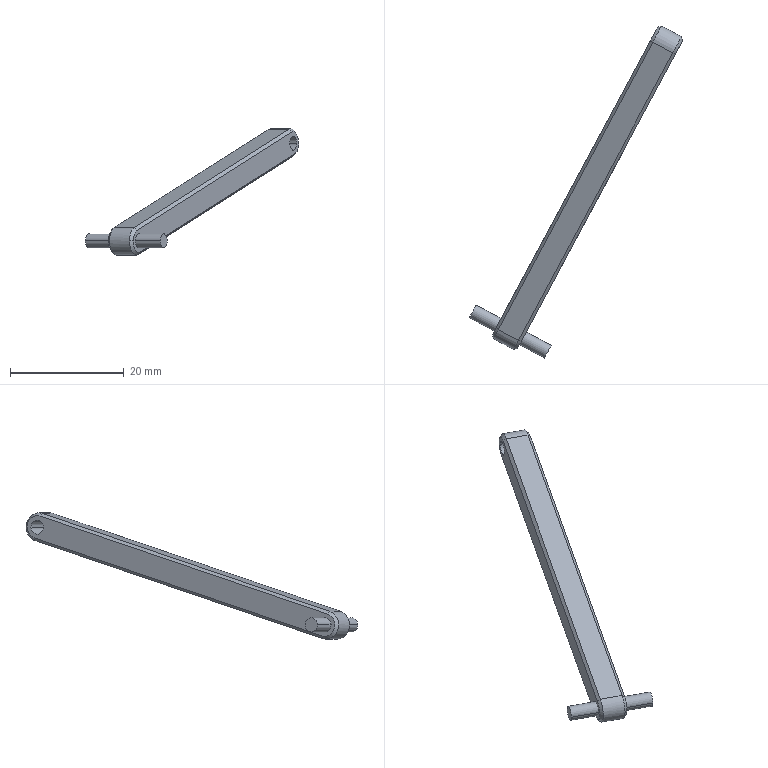Part | SolidWorks | features Revolution 2, Chamfer 1, Extrusion 1, HoleWzd 1 | 1 solid | 25 faces | box 37.545 x 58.428 x 22.236 mm | volume 1589 mm3 | plane 10 | cylinder 9 | cone 6 | commonest cylinder face diameters 2.5 x6 5 x3
STEP:
#1=CARTESIAN_POINT('',(-5.347,-33.041,-248.108));
#2=VERTEX_POINT('',#1);
#3=CARTESIAN_POINT('',(-6.022,-34.297,-250.024));
#4=VERTEX_POINT('',#3);
#5=CARTESIAN_POINT('',(-6.294,-34.803,-248.108));
#6=DIRECTION('',(-0.8809,0.4732,0.));
#7=DIRECTION('',(0.4732,0.8809,0.));
#8=AXIS2_PLACEMENT_3D('',#5,#6,#7);
#9=CIRCLE('',#8,2.);
#10=EDGE_CURVE('',#2,#4,#9,.T.);
#11=ORIENTED_EDGE('',*,*,#10,.F.);
#12=CARTESIAN_POINT('',(-4.67,-32.837,-248.108));
#13=VERTEX_POINT('',#12);
#14=CARTESIAN_POINT('',(-4.67,-32.837,-248.108));
#15=DIRECTION('',(0.9575,0.2883,0.));
#16=VECTOR('',#15,1000.);
#17=LINE('',#14,#16);
#18=EDGE_CURVE('',#2,#13,#17,.T.);
#19=ORIENTED_EDGE('',*,*,#18,.T.);
#20=CARTESIAN_POINT('',(-5.514,-34.407,-250.503));
#21=VERTEX_POINT('',#20);
#22=CARTESIAN_POINT('',(-5.853,-35.04,-248.108));
#23=DIRECTION('',(0.8809,-0.4732,0.));
#24=DIRECTION('',(0.4732,0.8809,0.));
#25=AXIS2_PLACEMENT_3D('',#22,#23,#24);
#26=CIRCLE('',#25,2.5);
#27=EDGE_CURVE('',#21,#13,#26,.T.);
#28=ORIENTED_EDGE('',*,*,#27,.F.);
#29=CARTESIAN_POINT('',(-6.022,-34.297,-250.024));
#30=DIRECTION('',(0.719,-0.1557,-0.6773));
#31=VECTOR('',#30,1000.);
#32=LINE('',#29,#31);
#33=EDGE_CURVE('',#4,#21,#32,.T.);
#34=ORIENTED_EDGE('',*,*,#33,.F.);
#35=EDGE_LOOP('',(#11,#19,#28,#34));
#36=FACE_OUTER_BOUND('',#35,.T.);
#37=CARTESIAN_POINT('',(-5.853,-35.04,-248.108));
#38=DIRECTION('',(0.8809,-0.4732,0.));
#39=DIRECTION('',(0.4732,0.8809,0.));
#40=AXIS2_PLACEMENT_3D('',#37,#38,#39);
#41=CONICAL_SURFACE('',#40,2.5,0.7854);
#42=ADVANCED_FACE('',(#36),#41,.T.);
#43=CARTESIAN_POINT('',(-30.033,-89.559,-265.344));
#44=VERTEX_POINT('',#43);
#45=CARTESIAN_POINT('',(-28.815,-87.291,-267.26));
#46=VERTEX_POINT('',#45);
#47=CARTESIAN_POINT('',(-29.087,-87.798,-265.344));
#48=DIRECTION('',(0.8809,-0.4732,0.));
#49=DIRECTION('',(0.4732,0.8809,0.));
#50=AXIS2_PLACEMENT_3D('',#47,#48,#49);
#51=CIRCLE('',#50,2.);
#52=EDGE_CURVE('',#44,#46,#51,.T.);
#53=ORIENTED_EDGE('',*,*,#52,.F.);
#54=CARTESIAN_POINT('',(-30.71,-89.763,-265.344));
#55=VERTEX_POINT('',#54);
#56=CARTESIAN_POINT('',(-30.033,-89.559,-265.344));
#57=DIRECTION('',(-0.9575,-0.2883,0.));
#58=VECTOR('',#57,1000.);
#59=LINE('',#56,#58);
#60=EDGE_CURVE('',#44,#55,#59,.T.);
#61=ORIENTED_EDGE('',*,*,#60,.T.);
#62=CARTESIAN_POINT('',(-29.187,-86.928,-267.739));
#63=VERTEX_POINT('',#62);
#64=CARTESIAN_POINT('',(-29.527,-87.561,-265.344));
#65=DIRECTION('',(-0.8809,0.4732,0.));
#66=DIRECTION('',(0.4732,0.8809,0.));
#67=AXIS2_PLACEMENT_3D('',#64,#65,#66);
#68=CIRCLE('',#67,2.5);
#69=EDGE_CURVE('',#63,#55,#68,.T.);
#70=ORIENTED_EDGE('',*,*,#69,.F.);
#71=CARTESIAN_POINT('',(-28.815,-87.291,-267.26));
#72=DIRECTION('',(-0.5268,0.5136,-0.6773));
#73=VECTOR('',#72,1000.);
#74=LINE('',#71,#73);
#75=EDGE_CURVE('',#46,#63,#74,.T.);
#76=ORIENTED_EDGE('',*,*,#75,.F.);
#77=EDGE_LOOP('',(#53,#61,#70,#76));
#78=FACE_OUTER_BOUND('',#77,.T.);
#79=CARTESIAN_POINT('',(-29.087,-87.798,-265.344));
#80=DIRECTION('',(-0.8809,0.4732,0.));
#81=DIRECTION('',(-0.4732,-0.8809,0.));
#82=AXIS2_PLACEMENT_3D('',#79,#80,#81);
#83=CONICAL_SURFACE('',#82,2.,0.7854);
#84=ADVANCED_FACE('',(#78),#83,.T.);
#85=CARTESIAN_POINT('',(-2.481,-38.27,-248.108));
#86=VERTEX_POINT('',#85);
#87=CARTESIAN_POINT('',(-1.298,-36.068,-248.108));
#88=VERTEX_POINT('',#87);
#89=CARTESIAN_POINT('',(-1.889,-37.169,-248.108));
#90=DIRECTION('',(0.8809,-0.4732,0.));
#91=DIRECTION('',(0.4732,0.8809,0.));
#92=AXIS2_PLACEMENT_3D('',#89,#90,#91);
#93=CIRCLE('',#92,1.25);
#94=EDGE_CURVE('',#86,#88,#93,.T.);
#95=ORIENTED_EDGE('',*,*,#94,.T.);
#96=CARTESIAN_POINT('',(-5.702,-33.702,-248.108));
#97=VERTEX_POINT('',#96);
#98=CARTESIAN_POINT('',(-5.702,-33.702,-248.108));
#99=DIRECTION('',(-0.8809,0.4732,0.));
#100=VECTOR('',#99,1000.);
#101=LINE('',#98,#100);
#102=EDGE_CURVE('',#88,#97,#101,.T.);
#103=ORIENTED_EDGE('',*,*,#102,.T.);
#104=CARTESIAN_POINT('',(-6.885,-35.904,-248.108));
#105=VERTEX_POINT('',#104);
#106=CARTESIAN_POINT('',(-6.294,-34.803,-248.108));
#107=DIRECTION('',(-0.8809,0.4732,0.));
#108=DIRECTION('',(-0.4732,-0.8809,0.));
#109=AXIS2_PLACEMENT_3D('',#106,#107,#108);
#110=CIRCLE('',#109,1.25);
#111=EDGE_CURVE('',#97,#105,#110,.T.);
#112=ORIENTED_EDGE('',*,*,#111,.T.);
#113=CARTESIAN_POINT('',(-6.885,-35.904,-248.108));
#114=DIRECTION('',(-0.8809,0.4732,0.));
#115=VECTOR('',#114,1000.);
#116=LINE('',#113,#115);
#117=EDGE_CURVE('',#86,#105,#116,.T.);
#118=ORIENTED_EDGE('',*,*,#117,.F.);
#119=EDGE_LOOP('',(#95,#103,#112,#118));
#120=FACE_OUTER_BOUND('',#119,.T.);
#121=CARTESIAN_POINT('',(-6.294,-34.803,-248.108));
#122=DIRECTION('',(-0.8809,0.4732,0.));
#123=DIRECTION('',(-0.4732,-0.8809,0.));
#124=AXIS2_PLACEMENT_3D('',#121,#122,#123);
#125=CYLINDRICAL_SURFACE('',#124,1.25);
#126=ADVANCED_FACE('',(#120),#125,.F.);
#127=CARTESIAN_POINT('',(-28.495,-86.696,-265.344));
#128=VERTEX_POINT('',#127);
#129=CARTESIAN_POINT('',(-29.678,-88.899,-265.344));
#130=VERTEX_POINT('',#129);
#131=CARTESIAN_POINT('',(-29.087,-87.798,-265.344));
#132=DIRECTION('',(0.8809,-0.4732,0.));
#133=DIRECTION('',(0.4732,0.8809,0.));
#134=AXIS2_PLACEMENT_3D('',#131,#132,#133);
#135=CIRCLE('',#134,1.25);
#136=EDGE_CURVE('',#128,#130,#135,.T.);
#137=ORIENTED_EDGE('',*,*,#136,.T.);
#138=CARTESIAN_POINT('',(-25.274,-91.265,-265.344));
#139=VERTEX_POINT('',#138);
#140=CARTESIAN_POINT('',(-28.692,-89.429,-265.344));
#141=DIRECTION('',(0.8809,-0.4732,0.));
#142=VECTOR('',#141,1000.);
#143=LINE('',#140,#142);
#144=EDGE_CURVE('',#130,#139,#143,.T.);
#145=ORIENTED_EDGE('',*,*,#144,.T.);
#146=CARTESIAN_POINT('',(-24.09,-89.063,-265.344));
#147=VERTEX_POINT('',#146);
#148=CARTESIAN_POINT('',(-24.682,-90.164,-265.344));
#149=DIRECTION('',(0.8809,-0.4732,0.));
#150=DIRECTION('',(0.4732,0.8809,0.));
#151=AXIS2_PLACEMENT_3D('',#148,#149,#150);
#152=CIRCLE('',#151,1.25);
#153=EDGE_CURVE('',#147,#139,#152,.T.);
#154=ORIENTED_EDGE('',*,*,#153,.F.);
#155=CARTESIAN_POINT('',(-27.509,-87.226,-265.344));
#156=DIRECTION('',(0.8809,-0.4732,0.));
#157=VECTOR('',#156,1000.);
#158=LINE('',#155,#157);
#159=EDGE_CURVE('',#128,#147,#158,.T.);
#160=ORIENTED_EDGE('',*,*,#159,.F.);
#161=EDGE_LOOP('',(#137,#145,#154,#160));
#162=FACE_OUTER_BOUND('',#161,.T.);
#163=CARTESIAN_POINT('',(-28.1,-88.327,-265.344));
#164=DIRECTION('',(0.8809,-0.4732,0.));
#165=DIRECTION('',(0.4732,0.8809,0.));
#166=AXIS2_PLACEMENT_3D('',#163,#164,#165);
#167=CYLINDRICAL_SURFACE('',#166,1.25);
#168=ADVANCED_FACE('',(#162),#167,.T.);
#169=CARTESIAN_POINT('',(-37.304,-81.964,-265.344));
#170=VERTEX_POINT('',#169);
#171=CARTESIAN_POINT('',(-38.488,-84.166,-265.344));
#172=VERTEX_POINT('',#171);
#173=CARTESIAN_POINT('',(-37.896,-83.065,-265.344));
#174=DIRECTION('',(0.8809,-0.4732,0.));
#175=DIRECTION('',(0.4732,0.8809,0.));
#176=AXIS2_PLACEMENT_3D('',#173,#174,#175);
#177=CIRCLE('',#176,1.25);
#178=EDGE_CURVE('',#170,#172,#177,.T.);
#179=ORIENTED_EDGE('',*,*,#178,.T.);
#180=CARTESIAN_POINT('',(-34.083,-86.532,-265.344));
#181=VERTEX_POINT('',#180);
#182=CARTESIAN_POINT('',(-37.501,-84.696,-265.344));
#183=DIRECTION('',(0.8809,-0.4732,0.));
#184=VECTOR('',#183,1000.);
#185=LINE('',#182,#184);
#186=EDGE_CURVE('',#172,#181,#185,.T.);
#187=ORIENTED_EDGE('',*,*,#186,.T.);
#188=CARTESIAN_POINT('',(-32.9,-84.33,-265.344));
#189=VERTEX_POINT('',#188);
#190=CARTESIAN_POINT('',(-33.491,-85.431,-265.344));
#191=DIRECTION('',(0.8809,-0.4732,0.));
#192=DIRECTION('',(0.4732,0.8809,0.));
#193=AXIS2_PLACEMENT_3D('',#190,#191,#192);
#194=CIRCLE('',#193,1.25);
#195=EDGE_CURVE('',#189,#181,#194,.T.);
#196=ORIENTED_EDGE('',*,*,#195,.F.);
#197=CARTESIAN_POINT('',(-36.318,-82.494,-265.344));
#198=DIRECTION('',(0.8809,-0.4732,0.));
#199=VECTOR('',#198,1000.);
#200=LINE('',#197,#199);
#201=EDGE_CURVE('',#170,#189,#200,.T.);
#202=ORIENTED_EDGE('',*,*,#201,.F.);
#203=EDGE_LOOP('',(#179,#187,#196,#202));
#204=FACE_OUTER_BOUND('',#203,.T.);
#205=CARTESIAN_POINT('',(-36.91,-83.595,-265.344));
#206=DIRECTION('',(0.8809,-0.4732,0.));
#207=DIRECTION('',(0.4732,0.8809,0.));
#208=AXIS2_PLACEMENT_3D('',#205,#206,#207);
#209=CYLINDRICAL_SURFACE('',#208,1.25);
#210=ADVANCED_FACE('',(#204),#209,.T.);
#211=ORIENTED_EDGE('',*,*,#27,.T.);
#212=CARTESIAN_POINT('',(-1.147,-34.73,-248.108));
#213=VERTEX_POINT('',#212);
#214=CARTESIAN_POINT('',(-5.111,-32.601,-248.108));
#215=DIRECTION('',(0.8809,-0.4732,0.));
#216=VECTOR('',#215,1000.);
#217=LINE('',#214,#216);
#218=EDGE_CURVE('',#13,#213,#217,.T.);
#219=ORIENTED_EDGE('',*,*,#218,.T.);
#220=CARTESIAN_POINT('',(-1.99,-36.3,-250.503));
#221=VERTEX_POINT('',#220);
#222=CARTESIAN_POINT('',(-2.33,-36.933,-248.108));
#223=DIRECTION('',(-0.8809,0.4732,0.));
#224=DIRECTION('',(0.4732,0.8809,0.));
#225=AXIS2_PLACEMENT_3D('',#222,#223,#224);
#226=CIRCLE('',#225,2.5);
#227=EDGE_CURVE('',#213,#221,#226,.T.);
#228=ORIENTED_EDGE('',*,*,#227,.T.);
#229=CARTESIAN_POINT('',(-5.954,-34.17,-250.503));
#230=DIRECTION('',(0.8809,-0.4732,0.));
#231=VECTOR('',#230,1000.);
#232=LINE('',#229,#231);
#233=EDGE_CURVE('',#21,#221,#232,.T.);
#234=ORIENTED_EDGE('',*,*,#233,.F.);
#235=EDGE_LOOP('',(#211,#219,#228,#234));
#236=FACE_OUTER_BOUND('',#235,.T.);
#237=CARTESIAN_POINT('',(-6.294,-34.803,-248.108));
#238=DIRECTION('',(0.8809,-0.4732,0.));
#239=DIRECTION('',(0.4732,0.8809,0.));
#240=AXIS2_PLACEMENT_3D('',#237,#238,#239);
#241=CYLINDRICAL_SURFACE('',#240,2.5);
#242=ADVANCED_FACE('',(#236),#241,.T.);
#243=CARTESIAN_POINT('',(-32.711,-85.035,-267.739));
#244=VERTEX_POINT('',#243);
#245=CARTESIAN_POINT('',(-33.151,-84.799,-267.739));
#246=DIRECTION('',(0.8809,-0.4732,0.));
#247=VECTOR('',#246,1000.);
#248=LINE('',#245,#247);
#249=EDGE_CURVE('',#244,#63,#248,.T.);
#250=ORIENTED_EDGE('',*,*,#249,.T.);
#251=ORIENTED_EDGE('',*,*,#69,.T.);
#252=CARTESIAN_POINT('',(-29.867,-88.194,-262.949));
#253=VERTEX_POINT('',#252);
#254=CARTESIAN_POINT('',(-29.527,-87.561,-265.344));
#255=DIRECTION('',(-0.8809,0.4732,0.));
#256=DIRECTION('',(0.4732,0.8809,0.));
#257=AXIS2_PLACEMENT_3D('',#254,#255,#256);
#258=CIRCLE('',#257,2.5);
#259=EDGE_CURVE('',#55,#253,#258,.T.);
#260=ORIENTED_EDGE('',*,*,#259,.T.);
#261=CARTESIAN_POINT('',(-33.391,-86.301,-262.949));
#262=VERTEX_POINT('',#261);
#263=CARTESIAN_POINT('',(-33.831,-86.064,-262.949));
#264=DIRECTION('',(0.8809,-0.4732,0.));
#265=VECTOR('',#264,1000.);
#266=LINE('',#263,#265);
#267=EDGE_CURVE('',#262,#253,#266,.T.);
#268=ORIENTED_EDGE('',*,*,#267,.F.);
#269=CARTESIAN_POINT('',(-33.051,-85.668,-265.344));
#270=DIRECTION('',(0.8809,-0.4732,0.));
#271=DIRECTION('',(0.4732,0.8809,0.));
#272=AXIS2_PLACEMENT_3D('',#269,#270,#271);
#273=CIRCLE('',#272,2.5);
#274=EDGE_CURVE('',#262,#244,#273,.T.);
#275=ORIENTED_EDGE('',*,*,#274,.T.);
#276=EDGE_LOOP('',(#250,#251,#260,#268,#275));
#277=FACE_OUTER_BOUND('',#276,.T.);
#278=CARTESIAN_POINT('',(-33.491,-85.431,-265.344));
#279=DIRECTION('',(0.8809,-0.4732,0.));
#280=DIRECTION('',(0.4732,0.8809,0.));
#281=AXIS2_PLACEMENT_3D('',#278,#279,#280);
#282=CYLINDRICAL_SURFACE('',#281,2.5);
#283=ADVANCED_FACE('',(#277),#282,.T.);
#284=ORIENTED_EDGE('',*,*,#267,.T.);
#285=CARTESIAN_POINT('',(-2.67,-37.565,-245.714));
#286=VERTEX_POINT('',#285);
#287=CARTESIAN_POINT('',(-2.67,-37.565,-245.714));
#288=DIRECTION('',(0.4533,0.8438,0.2873));
#289=VECTOR('',#288,1000.);
#290=LINE('',#287,#289);
#291=EDGE_CURVE('',#253,#286,#290,.T.);
#292=ORIENTED_EDGE('',*,*,#291,.T.);
#293=CARTESIAN_POINT('',(-6.193,-35.672,-245.714));
#294=VERTEX_POINT('',#293);
#295=CARTESIAN_POINT('',(-6.634,-35.436,-245.714));
#296=DIRECTION('',(0.8809,-0.4732,0.));
#297=VECTOR('',#296,1000.);
#298=LINE('',#295,#297);
#299=EDGE_CURVE('',#294,#286,#298,.T.);
#300=ORIENTED_EDGE('',*,*,#299,.F.);
#301=CARTESIAN_POINT('',(-33.391,-86.301,-262.949));
#302=DIRECTION('',(-0.4533,-0.8438,-0.2873));
#303=VECTOR('',#302,1000.);
#304=LINE('',#301,#303);
#305=EDGE_CURVE('',#294,#262,#304,.T.);
#306=ORIENTED_EDGE('',*,*,#305,.T.);
#307=EDGE_LOOP('',(#284,#292,#300,#306));
#308=FACE_OUTER_BOUND('',#307,.T.);
#309=CARTESIAN_POINT('',(-6.634,-35.436,-245.714));
#310=DIRECTION('',(-0.1359,-0.2531,0.9579));
#311=DIRECTION('',(0.,-0.9668,-0.2554));
#312=AXIS2_PLACEMENT_3D('',#309,#310,#311);
#313=PLANE('',#312);
#314=ADVANCED_FACE('',(#308),#313,.T.);
#315=ORIENTED_EDGE('',*,*,#218,.F.);
#316=CARTESIAN_POINT('',(-5.853,-35.04,-248.108));
#317=DIRECTION('',(0.8809,-0.4732,0.));
#318=DIRECTION('',(0.4732,0.8809,0.));
#319=AXIS2_PLACEMENT_3D('',#316,#317,#318);
#320=CIRCLE('',#319,2.5);
#321=EDGE_CURVE('',#13,#294,#320,.T.);
#322=ORIENTED_EDGE('',*,*,#321,.T.);
#323=ORIENTED_EDGE('',*,*,#299,.T.);
#324=CARTESIAN_POINT('',(-2.33,-36.933,-248.108));
#325=DIRECTION('',(-0.8809,0.4732,0.));
#326=DIRECTION('',(0.4732,0.8809,0.));
#327=AXIS2_PLACEMENT_3D('',#324,#325,#326);
#328=CIRCLE('',#327,2.5);
#329=EDGE_CURVE('',#286,#213,#328,.T.);
#330=ORIENTED_EDGE('',*,*,#329,.T.);
#331=EDGE_LOOP('',(#315,#322,#323,#330));
#332=FACE_OUTER_BOUND('',#331,.T.);
#333=CARTESIAN_POINT('',(-6.294,-34.803,-248.108));
#334=DIRECTION('',(0.8809,-0.4732,0.));
#335=DIRECTION('',(0.4732,0.8809,0.));
#336=AXIS2_PLACEMENT_3D('',#333,#334,#335);
#337=CYLINDRICAL_SURFACE('',#336,2.5);
#338=ADVANCED_FACE('',(#332),#337,.T.);
#339=ORIENTED_EDGE('',*,*,#233,.T.);
#340=CARTESIAN_POINT('',(-29.187,-86.928,-267.739));
#341=DIRECTION('',(-0.4533,-0.8438,-0.2873));
#342=VECTOR('',#341,1000.);
#343=LINE('',#340,#342);
#344=EDGE_CURVE('',#221,#63,#343,.T.);
#345=ORIENTED_EDGE('',*,*,#344,.T.);
#346=ORIENTED_EDGE('',*,*,#249,.F.);
#347=CARTESIAN_POINT('',(-5.514,-34.407,-250.503));
#348=DIRECTION('',(0.4533,0.8438,0.2873));
#349=VECTOR('',#348,1000.);
#350=LINE('',#347,#349);
#351=EDGE_CURVE('',#244,#21,#350,.T.);
#352=ORIENTED_EDGE('',*,*,#351,.T.);
#353=EDGE_LOOP('',(#339,#345,#346,#352));
#354=FACE_OUTER_BOUND('',#353,.T.);
#355=CARTESIAN_POINT('',(-33.151,-84.799,-267.739));
#356=DIRECTION('',(0.1359,0.2531,-0.9579));
#357=DIRECTION('',(0.,0.9668,0.2554));
#358=AXIS2_PLACEMENT_3D('',#355,#356,#357);
#359=PLANE('',#358);
#360=ADVANCED_FACE('',(#354),#359,.T.);
#361=CARTESIAN_POINT('',(-6.566,-35.309,-246.192));
#362=VERTEX_POINT('',#361);
#363=CARTESIAN_POINT('',(-6.294,-34.803,-248.108));
#364=DIRECTION('',(-0.8809,0.4732,0.));
#365=DIRECTION('',(0.4732,0.8809,0.));
#366=AXIS2_PLACEMENT_3D('',#363,#364,#365);
#367=CIRCLE('',#366,2.);
#368=EDGE_CURVE('',#362,#2,#367,.T.);
#369=ORIENTED_EDGE('',*,*,#368,.T.);
#370=ORIENTED_EDGE('',*,*,#10,.T.);
#371=CARTESIAN_POINT('',(-33.219,-84.925,-267.26));
#372=VERTEX_POINT('',#371);
#373=CARTESIAN_POINT('',(-33.219,-84.925,-267.26));
#374=DIRECTION('',(-0.4533,-0.8438,-0.2873));
#375=VECTOR('',#374,1000.);
#376=LINE('',#373,#375);
#377=EDGE_CURVE('',#4,#372,#376,.T.);
#378=ORIENTED_EDGE('',*,*,#377,.T.);
#379=CARTESIAN_POINT('',(-33.763,-85.937,-263.428));
#380=VERTEX_POINT('',#379);
#381=CARTESIAN_POINT('',(-33.491,-85.431,-265.344));
#382=DIRECTION('',(-0.8809,0.4732,0.));
#383=DIRECTION('',(0.4732,0.8809,0.));
#384=AXIS2_PLACEMENT_3D('',#381,#382,#383);
#385=CIRCLE('',#384,2.);
#386=EDGE_CURVE('',#372,#380,#385,.T.);
#387=ORIENTED_EDGE('',*,*,#386,.T.);
#388=CARTESIAN_POINT('',(-6.566,-35.309,-246.192));
#389=DIRECTION('',(0.4533,0.8438,0.2873));
#390=VECTOR('',#389,1000.);
#391=LINE('',#388,#390);
#392=EDGE_CURVE('',#380,#362,#391,.T.);
#393=ORIENTED_EDGE('',*,*,#392,.T.);
#394=EDGE_LOOP('',(#369,#370,#378,#387,#393));
#395=FACE_OUTER_BOUND('',#394,.T.);
#396=CARTESIAN_POINT('',(-6.294,-34.803,-248.108));
#397=DIRECTION('',(-0.8809,0.4732,0.));
#398=DIRECTION('',(-0.4732,-0.8809,0.));
#399=AXIS2_PLACEMENT_3D('',#396,#397,#398);
#400=CIRCLE('',#399,1.25);
#401=EDGE_CURVE('',#105,#97,#400,.T.);
#402=ORIENTED_EDGE('',*,*,#401,.F.);
#403=ORIENTED_EDGE('',*,*,#111,.F.);
#404=EDGE_LOOP('',(#402,#403));
#405=FACE_BOUND('',#404,.T.);
#406=ORIENTED_EDGE('',*,*,#195,.T.);
#407=CARTESIAN_POINT('',(-33.491,-85.431,-265.344));
#408=DIRECTION('',(0.8809,-0.4732,0.));
#409=DIRECTION('',(0.4732,0.8809,0.));
#410=AXIS2_PLACEMENT_3D('',#407,#408,#409);
#411=CIRCLE('',#410,1.25);
#412=EDGE_CURVE('',#181,#189,#411,.T.);
#413=ORIENTED_EDGE('',*,*,#412,.T.);
#414=EDGE_LOOP('',(#406,#413));
#415=FACE_BOUND('',#414,.T.);
#416=CARTESIAN_POINT('',(-33.491,-85.431,-265.344));
#417=DIRECTION('',(0.8809,-0.4732,0.));
#418=DIRECTION('',(0.4732,0.8809,0.));
#419=AXIS2_PLACEMENT_3D('',#416,#417,#418);
#420=PLANE('',#419);
#421=ADVANCED_FACE('',(#395,#405,#415),#420,.F.);
#422=CARTESIAN_POINT('',(-1.617,-36.663,-250.024));
#423=VERTEX_POINT('',#422);
#424=CARTESIAN_POINT('',(-28.815,-87.291,-267.26));
#425=DIRECTION('',(0.4533,0.8438,0.2873));
#426=VECTOR('',#425,1000.);
#427=LINE('',#424,#426);
#428=EDGE_CURVE('',#46,#423,#427,.T.);
#429=ORIENTED_EDGE('',*,*,#428,.T.);
#430=CARTESIAN_POINT('',(-2.161,-37.675,-246.192));
#431=VERTEX_POINT('',#430);
#432=CARTESIAN_POINT('',(-1.889,-37.169,-248.108));
#433=DIRECTION('',(0.8809,-0.4732,0.));
#434=DIRECTION('',(0.4732,0.8809,0.));
#435=AXIS2_PLACEMENT_3D('',#432,#433,#434);
#436=CIRCLE('',#435,2.);
#437=EDGE_CURVE('',#423,#431,#436,.T.);
#438=ORIENTED_EDGE('',*,*,#437,.T.);
#439=CARTESIAN_POINT('',(-29.359,-88.304,-263.428));
#440=VERTEX_POINT('',#439);
#441=CARTESIAN_POINT('',(-29.359,-88.304,-263.428));
#442=DIRECTION('',(-0.4533,-0.8438,-0.2873));
#443=VECTOR('',#442,1000.);
#444=LINE('',#441,#443);
#445=EDGE_CURVE('',#431,#440,#444,.T.);
#446=ORIENTED_EDGE('',*,*,#445,.T.);
#447=CARTESIAN_POINT('',(-29.087,-87.798,-265.344));
#448=DIRECTION('',(0.8809,-0.4732,0.));
#449=DIRECTION('',(0.4732,0.8809,0.));
#450=AXIS2_PLACEMENT_3D('',#447,#448,#449);
#451=CIRCLE('',#450,2.);
#452=EDGE_CURVE('',#440,#44,#451,.T.);
#453=ORIENTED_EDGE('',*,*,#452,.T.);
#454=ORIENTED_EDGE('',*,*,#52,.T.);
#455=EDGE_LOOP('',(#429,#438,#446,#453,#454));
#456=FACE_OUTER_BOUND('',#455,.T.);
#457=ORIENTED_EDGE('',*,*,#94,.F.);
#458=CARTESIAN_POINT('',(-1.889,-37.169,-248.108));
#459=DIRECTION('',(0.8809,-0.4732,0.));
#460=DIRECTION('',(0.4732,0.8809,0.));
#461=AXIS2_PLACEMENT_3D('',#458,#459,#460);
#462=CIRCLE('',#461,1.25);
#463=EDGE_CURVE('',#88,#86,#462,.T.);
#464=ORIENTED_EDGE('',*,*,#463,.F.);
#465=EDGE_LOOP('',(#457,#464));
#466=FACE_BOUND('',#465,.T.);
#467=ORIENTED_EDGE('',*,*,#136,.F.);
#468=CARTESIAN_POINT('',(-29.087,-87.798,-265.344));
#469=DIRECTION('',(0.8809,-0.4732,0.));
#470=DIRECTION('',(0.4732,0.8809,0.));
#471=AXIS2_PLACEMENT_3D('',#468,#469,#470);
#472=CIRCLE('',#471,1.25);
#473=EDGE_CURVE('',#130,#128,#472,.T.);
#474=ORIENTED_EDGE('',*,*,#473,.F.);
#475=EDGE_LOOP('',(#467,#474));
#476=FACE_BOUND('',#475,.T.);
#477=CARTESIAN_POINT('',(-29.087,-87.798,-265.344));
#478=DIRECTION('',(0.8809,-0.4732,0.));
#479=DIRECTION('',(0.4732,0.8809,0.));
#480=AXIS2_PLACEMENT_3D('',#477,#478,#479);
#481=PLANE('',#480);
#482=ADVANCED_FACE('',(#456,#466,#476),#481,.T.);
#483=ORIENTED_EDGE('',*,*,#186,.F.);
#484=CARTESIAN_POINT('',(-37.896,-83.065,-265.344));
#485=DIRECTION('',(0.8809,-0.4732,0.));
#486=DIRECTION('',(0.4732,0.8809,0.));
#487=AXIS2_PLACEMENT_3D('',#484,#485,#486);
#488=CIRCLE('',#487,1.25);
#489=EDGE_CURVE('',#172,#170,#488,.T.);
#490=ORIENTED_EDGE('',*,*,#489,.T.);
#491=ORIENTED_EDGE('',*,*,#201,.T.);
#492=ORIENTED_EDGE('',*,*,#412,.F.);
#493=EDGE_LOOP('',(#483,#490,#491,#492));
#494=FACE_OUTER_BOUND('',#493,.T.);
#495=CARTESIAN_POINT('',(-36.91,-83.595,-265.344));
#496=DIRECTION('',(0.8809,-0.4732,0.));
#497=DIRECTION('',(0.4732,0.8809,0.));
#498=AXIS2_PLACEMENT_3D('',#495,#496,#497);
#499=CYLINDRICAL_SURFACE('',#498,1.25);
#500=ADVANCED_FACE('',(#494),#499,.T.);
#501=ORIENTED_EDGE('',*,*,#178,.F.);
#502=ORIENTED_EDGE('',*,*,#489,.F.);
#503=EDGE_LOOP('',(#501,#502));
#504=FACE_OUTER_BOUND('',#503,.T.);
#505=CARTESIAN_POINT('',(-37.304,-81.964,-265.344));
#506=DIRECTION('',(-0.8809,0.4732,0.));
#507=DIRECTION('',(-0.4732,-0.8809,0.));
#508=AXIS2_PLACEMENT_3D('',#505,#506,#507);
#509=PLANE('',#508);
#510=ADVANCED_FACE('',(#504),#509,.T.);
#511=ORIENTED_EDGE('',*,*,#144,.F.);
#512=ORIENTED_EDGE('',*,*,#473,.T.);
#513=ORIENTED_EDGE('',*,*,#159,.T.);
#514=CARTESIAN_POINT('',(-24.682,-90.164,-265.344));
#515=DIRECTION('',(0.8809,-0.4732,0.));
#516=DIRECTION('',(0.4732,0.8809,0.));
#517=AXIS2_PLACEMENT_3D('',#514,#515,#516);
#518=CIRCLE('',#517,1.25);
#519=EDGE_CURVE('',#139,#147,#518,.T.);
#520=ORIENTED_EDGE('',*,*,#519,.F.);
#521=EDGE_LOOP('',(#511,#512,#513,#520));
#522=FACE_OUTER_BOUND('',#521,.T.);
#523=CARTESIAN_POINT('',(-28.1,-88.327,-265.344));
#524=DIRECTION('',(0.8809,-0.4732,0.));
#525=DIRECTION('',(0.4732,0.8809,0.));
#526=AXIS2_PLACEMENT_3D('',#523,#524,#525);
#527=CYLINDRICAL_SURFACE('',#526,1.25);
#528=ADVANCED_FACE('',(#522),#527,.T.);
#529=ORIENTED_EDGE('',*,*,#153,.T.);
#530=ORIENTED_EDGE('',*,*,#519,.T.);
#531=EDGE_LOOP('',(#529,#530));
#532=FACE_OUTER_BOUND('',#531,.T.);
#533=CARTESIAN_POINT('',(-24.682,-90.164,-265.344));
#534=DIRECTION('',(0.8809,-0.4732,0.));
#535=DIRECTION('',(0.4732,0.8809,0.));
#536=AXIS2_PLACEMENT_3D('',#533,#534,#535);
#537=PLANE('',#536);
#538=ADVANCED_FACE('',(#532),#537,.T.);
#539=ORIENTED_EDGE('',*,*,#102,.F.);
#540=ORIENTED_EDGE('',*,*,#463,.T.);
#541=ORIENTED_EDGE('',*,*,#117,.T.);
#542=ORIENTED_EDGE('',*,*,#401,.T.);
#543=EDGE_LOOP('',(#539,#540,#541,#542));
#544=FACE_OUTER_BOUND('',#543,.T.);
#545=CARTESIAN_POINT('',(-6.294,-34.803,-248.108));
#546=DIRECTION('',(-0.8809,0.4732,0.));
#547=DIRECTION('',(-0.4732,-0.8809,0.));
#548=AXIS2_PLACEMENT_3D('',#545,#546,#547);
#549=CYLINDRICAL_SURFACE('',#548,1.25);
#550=ADVANCED_FACE('',(#544),#549,.F.);
#551=ORIENTED_EDGE('',*,*,#60,.F.);
#552=ORIENTED_EDGE('',*,*,#452,.F.);
#553=CARTESIAN_POINT('',(-29.867,-88.194,-262.949));
#554=DIRECTION('',(0.719,-0.1557,-0.6773));
#555=VECTOR('',#554,1000.);
#556=LINE('',#553,#555);
#557=EDGE_CURVE('',#253,#440,#556,.T.);
#558=ORIENTED_EDGE('',*,*,#557,.F.);
#559=ORIENTED_EDGE('',*,*,#259,.F.);
#560=EDGE_LOOP('',(#551,#552,#558,#559));
#561=FACE_OUTER_BOUND('',#560,.T.);
#562=CARTESIAN_POINT('',(-29.087,-87.798,-265.344));
#563=DIRECTION('',(-0.8809,0.4732,0.));
#564=DIRECTION('',(-0.4732,-0.8809,0.));
#565=AXIS2_PLACEMENT_3D('',#562,#563,#564);
#566=CONICAL_SURFACE('',#565,2.,0.7854);
#567=ADVANCED_FACE('',(#561),#566,.T.);
#568=ORIENTED_EDGE('',*,*,#75,.T.);
#569=ORIENTED_EDGE('',*,*,#344,.F.);
#570=CARTESIAN_POINT('',(-1.617,-36.663,-250.024));
#571=DIRECTION('',(-0.5268,0.5136,-0.6773));
#572=VECTOR('',#571,1000.);
#573=LINE('',#570,#572);
#574=EDGE_CURVE('',#423,#221,#573,.T.);
#575=ORIENTED_EDGE('',*,*,#574,.F.);
#576=ORIENTED_EDGE('',*,*,#428,.F.);
#577=EDGE_LOOP('',(#568,#569,#575,#576));
#578=FACE_OUTER_BOUND('',#577,.T.);
#579=CARTESIAN_POINT('',(-28.815,-87.291,-267.26));
#580=DIRECTION('',(-0.719,0.1557,0.6773));
#581=DIRECTION('',(0.4533,0.8438,0.2873));
#582=AXIS2_PLACEMENT_3D('',#579,#580,#581);
#583=PLANE('',#582);
#584=ADVANCED_FACE('',(#578),#583,.F.);
#585=ORIENTED_EDGE('',*,*,#557,.T.);
#586=ORIENTED_EDGE('',*,*,#445,.F.);
#587=CARTESIAN_POINT('',(-2.67,-37.565,-245.714));
#588=DIRECTION('',(0.719,-0.1557,-0.6773));
#589=VECTOR('',#588,1000.);
#590=LINE('',#587,#589);
#591=EDGE_CURVE('',#286,#431,#590,.T.);
#592=ORIENTED_EDGE('',*,*,#591,.F.);
#593=ORIENTED_EDGE('',*,*,#291,.F.);
#594=EDGE_LOOP('',(#585,#586,#592,#593));
#595=FACE_OUTER_BOUND('',#594,.T.);
#596=CARTESIAN_POINT('',(-29.359,-88.304,-263.428));
#597=DIRECTION('',(-0.5268,0.5136,-0.6773));
#598=DIRECTION('',(-0.4533,-0.8438,-0.2873));
#599=AXIS2_PLACEMENT_3D('',#596,#597,#598);
#600=PLANE('',#599);
#601=ADVANCED_FACE('',(#595),#600,.F.);
#602=ORIENTED_EDGE('',*,*,#574,.T.);
#603=ORIENTED_EDGE('',*,*,#227,.F.);
#604=ORIENTED_EDGE('',*,*,#329,.F.);
#605=ORIENTED_EDGE('',*,*,#591,.T.);
#606=ORIENTED_EDGE('',*,*,#437,.F.);
#607=EDGE_LOOP('',(#602,#603,#604,#605,#606));
#608=FACE_OUTER_BOUND('',#607,.T.);
#609=CARTESIAN_POINT('',(-1.889,-37.169,-248.108));
#610=DIRECTION('',(-0.8809,0.4732,0.));
#611=DIRECTION('',(-0.4732,-0.8809,0.));
#612=AXIS2_PLACEMENT_3D('',#609,#610,#611);
#613=CONICAL_SURFACE('',#612,2.,0.7854);
#614=ADVANCED_FACE('',(#608),#613,.T.);
#615=CARTESIAN_POINT('',(-6.566,-35.309,-246.192));
#616=DIRECTION('',(0.5268,-0.5136,0.6773));
#617=VECTOR('',#616,1000.);
#618=LINE('',#615,#617);
#619=EDGE_CURVE('',#362,#294,#618,.T.);
#620=ORIENTED_EDGE('',*,*,#619,.F.);
#621=ORIENTED_EDGE('',*,*,#392,.F.);
#622=CARTESIAN_POINT('',(-33.391,-86.301,-262.949));
#623=DIRECTION('',(-0.5268,0.5136,-0.6773));
#624=VECTOR('',#623,1000.);
#625=LINE('',#622,#624);
#626=EDGE_CURVE('',#262,#380,#625,.T.);
#627=ORIENTED_EDGE('',*,*,#626,.F.);
#628=ORIENTED_EDGE('',*,*,#305,.F.);
#629=EDGE_LOOP('',(#620,#621,#627,#628));
#630=FACE_OUTER_BOUND('',#629,.T.);
#631=CARTESIAN_POINT('',(-6.193,-35.672,-245.714));
#632=DIRECTION('',(-0.719,0.1557,0.6773));
#633=DIRECTION('',(0.4533,0.8438,0.2873));
#634=AXIS2_PLACEMENT_3D('',#631,#632,#633);
#635=PLANE('',#634);
#636=ADVANCED_FACE('',(#630),#635,.T.);
#637=ORIENTED_EDGE('',*,*,#626,.T.);
#638=ORIENTED_EDGE('',*,*,#386,.F.);
#639=CARTESIAN_POINT('',(-32.711,-85.035,-267.739));
#640=DIRECTION('',(-0.719,0.1557,0.6773));
#641=VECTOR('',#640,1000.);
#642=LINE('',#639,#641);
#643=EDGE_CURVE('',#244,#372,#642,.T.);
#644=ORIENTED_EDGE('',*,*,#643,.F.);
#645=ORIENTED_EDGE('',*,*,#274,.F.);
#646=EDGE_LOOP('',(#637,#638,#644,#645));
#647=FACE_OUTER_BOUND('',#646,.T.);
#648=CARTESIAN_POINT('',(-33.051,-85.668,-265.344));
#649=DIRECTION('',(0.8809,-0.4732,0.));
#650=DIRECTION('',(0.4732,0.8809,0.));
#651=AXIS2_PLACEMENT_3D('',#648,#649,#650);
#652=CONICAL_SURFACE('',#651,2.5,0.7854);
#653=ADVANCED_FACE('',(#647),#652,.T.);
#654=ORIENTED_EDGE('',*,*,#18,.F.);
#655=ORIENTED_EDGE('',*,*,#368,.F.);
#656=ORIENTED_EDGE('',*,*,#619,.T.);
#657=ORIENTED_EDGE('',*,*,#321,.F.);
#658=EDGE_LOOP('',(#654,#655,#656,#657));
#659=FACE_OUTER_BOUND('',#658,.T.);
#660=CARTESIAN_POINT('',(-5.853,-35.04,-248.108));
#661=DIRECTION('',(0.8809,-0.4732,0.));
#662=DIRECTION('',(0.4732,0.8809,0.));
#663=AXIS2_PLACEMENT_3D('',#660,#661,#662);
#664=CONICAL_SURFACE('',#663,2.5,0.7854);
#665=ADVANCED_FACE('',(#659),#664,.T.);
#666=ORIENTED_EDGE('',*,*,#643,.T.);
#667=ORIENTED_EDGE('',*,*,#377,.F.);
#668=ORIENTED_EDGE('',*,*,#33,.T.);
#669=ORIENTED_EDGE('',*,*,#351,.F.);
#670=EDGE_LOOP('',(#666,#667,#668,#669));
#671=FACE_OUTER_BOUND('',#670,.T.);
#672=CARTESIAN_POINT('',(-32.711,-85.035,-267.739));
#673=DIRECTION('',(-0.5268,0.5136,-0.6773));
#674=DIRECTION('',(-0.4533,-0.8438,-0.2873));
#675=AXIS2_PLACEMENT_3D('',#672,#673,#674);
#676=PLANE('',#675);
#677=ADVANCED_FACE('',(#671),#676,.T.);
#678=CLOSED_SHELL('',(#42,#84,#126,#168,#210,#242,#283,#314,#338,#360,#421,#482,#500,#510,#528,#538,#550,#567,#584,#601,#614,#636,#653,#665,#677));
#679=MANIFOLD_SOLID_BREP('',#678);
#680=CARTESIAN_POINT('',(0.,0.,0.));
#681=DIRECTION('',(0.,0.,1.));
#682=DIRECTION('',(1.,0.,0.));
#683=AXIS2_PLACEMENT_3D('',#680,#681,#682);
#684=(LENGTH_UNIT()NAMED_UNIT(*)SI_UNIT(.MILLI.,.METRE.));
#685=UNCERTAINTY_MEASURE_WITH_UNIT(LENGTH_MEASURE(0.00001),#684,'','');
#686=(NAMED_UNIT(*)PLANE_ANGLE_UNIT()SI_UNIT($,.RADIAN.));
#687=(NAMED_UNIT(*)SI_UNIT($,.STERADIAN.)SOLID_ANGLE_UNIT());
#688=(GEOMETRIC_REPRESENTATION_CONTEXT(3)GLOBAL_UNCERTAINTY_ASSIGNED_CONTEXT((#685))GLOBAL_UNIT_ASSIGNED_CONTEXT((#684,#686,#687))REPRESENTATION_CONTEXT('',''));
#689=ADVANCED_BREP_SHAPE_REPRESENTATION('',(#679,#683),#688);